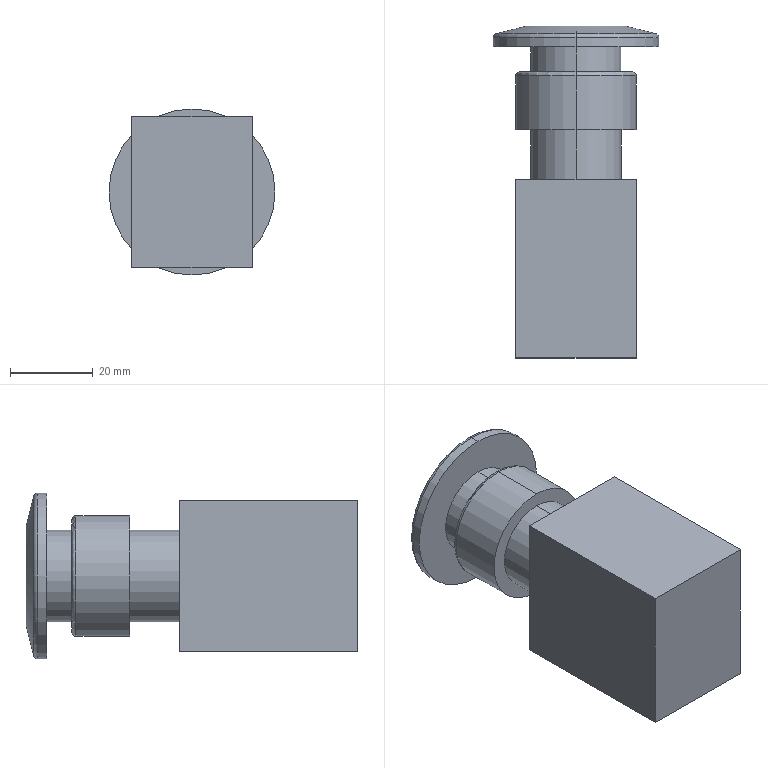Part | SolidWorks | features ICE 4, Extrusion 1, Fillet 1, RevCut 1 | 1 solid | 24 faces | box 40 x 80 x 40 mm | volume 67108 mm3 | plane 10 | cylinder 8 | torus 4 | cone 2 | commonest cylinder face diameters 22 x4 29 x2 40 x2
STEP:
#1=CARTESIAN_POINT('',(0.,-12.,-11.));
#2=VERTEX_POINT('',#1);
#3=CARTESIAN_POINT('',(0.,-12.,11.));
#4=VERTEX_POINT('',#3);
#5=CARTESIAN_POINT('',(0.,-12.,0.));
#6=DIRECTION('',(0.,-1.,0.));
#7=DIRECTION('',(0.,0.,-1.));
#8=AXIS2_PLACEMENT_3D('',#5,#6,#7);
#9=CIRCLE('',#8,11.);
#10=EDGE_CURVE('',#2,#4,#9,.T.);
#11=ORIENTED_EDGE('',*,*,#10,.F.);
#12=CARTESIAN_POINT('',(0.,0.,-11.));
#13=VERTEX_POINT('',#12);
#14=CARTESIAN_POINT('',(0.,-12.,-11.));
#15=DIRECTION('',(0.,1.,0.));
#16=VECTOR('',#15,1000.);
#17=LINE('',#14,#16);
#18=EDGE_CURVE('',#2,#13,#17,.T.);
#19=ORIENTED_EDGE('',*,*,#18,.T.);
#20=CARTESIAN_POINT('',(0.,0.,11.));
#21=VERTEX_POINT('',#20);
#22=CARTESIAN_POINT('',(0.,0.,0.));
#23=DIRECTION('',(0.,-1.,0.));
#24=DIRECTION('',(0.,0.,1.));
#25=AXIS2_PLACEMENT_3D('',#22,#23,#24);
#26=CIRCLE('',#25,11.);
#27=EDGE_CURVE('',#13,#21,#26,.T.);
#28=ORIENTED_EDGE('',*,*,#27,.T.);
#29=CARTESIAN_POINT('',(0.,-12.,11.));
#30=DIRECTION('',(0.,1.,0.));
#31=VECTOR('',#30,1000.);
#32=LINE('',#29,#31);
#33=EDGE_CURVE('',#4,#21,#32,.T.);
#34=ORIENTED_EDGE('',*,*,#33,.F.);
#35=EDGE_LOOP('',(#11,#19,#28,#34));
#36=FACE_OUTER_BOUND('',#35,.T.);
#37=CARTESIAN_POINT('',(0.,-12.,0.));
#38=DIRECTION('',(0.,1.,0.));
#39=DIRECTION('',(0.,0.,1.));
#40=AXIS2_PLACEMENT_3D('',#37,#38,#39);
#41=CYLINDRICAL_SURFACE('',#40,11.);
#42=ADVANCED_FACE('',(#36),#41,.T.);
#43=CARTESIAN_POINT('',(0.,22.219,-20.));
#44=VERTEX_POINT('',#43);
#45=CARTESIAN_POINT('',(0.,22.219,20.));
#46=VERTEX_POINT('',#45);
#47=CARTESIAN_POINT('',(0.,22.219,0.));
#48=DIRECTION('',(0.,-1.,0.));
#49=DIRECTION('',(0.,0.,1.));
#50=AXIS2_PLACEMENT_3D('',#47,#48,#49);
#51=CIRCLE('',#50,20.);
#52=EDGE_CURVE('',#44,#46,#51,.T.);
#53=ORIENTED_EDGE('',*,*,#52,.F.);
#54=CARTESIAN_POINT('',(0.,23.189,-19.243));
#55=VERTEX_POINT('',#54);
#56=CARTESIAN_POINT('',(0.,22.219,-19.));
#57=DIRECTION('',(1.,0.,0.));
#58=DIRECTION('',(0.,0.,-1.));
#59=AXIS2_PLACEMENT_3D('',#56,#57,#58);
#60=CIRCLE('',#59,1.);
#61=EDGE_CURVE('',#44,#55,#60,.T.);
#62=ORIENTED_EDGE('',*,*,#61,.T.);
#63=CARTESIAN_POINT('',(0.,23.189,19.243));
#64=VERTEX_POINT('',#63);
#65=CARTESIAN_POINT('',(0.,23.189,0.));
#66=DIRECTION('',(0.,1.,0.));
#67=DIRECTION('',(0.,0.,-1.));
#68=AXIS2_PLACEMENT_3D('',#65,#66,#67);
#69=CIRCLE('',#68,19.243);
#70=EDGE_CURVE('',#64,#55,#69,.T.);
#71=ORIENTED_EDGE('',*,*,#70,.F.);
#72=CARTESIAN_POINT('',(0.,22.219,19.));
#73=DIRECTION('',(-1.,0.,0.));
#74=DIRECTION('',(0.,0.,1.));
#75=AXIS2_PLACEMENT_3D('',#72,#73,#74);
#76=CIRCLE('',#75,1.);
#77=EDGE_CURVE('',#46,#64,#76,.T.);
#78=ORIENTED_EDGE('',*,*,#77,.F.);
#79=EDGE_LOOP('',(#53,#62,#71,#78));
#80=FACE_OUTER_BOUND('',#79,.T.);
#81=CARTESIAN_POINT('',(0.,22.219,0.));
#82=DIRECTION('',(0.,1.,0.));
#83=DIRECTION('',(0.,0.,1.));
#84=AXIS2_PLACEMENT_3D('',#81,#82,#83);
#85=TOROIDAL_SURFACE('',#84,19.,1.);
#86=ADVANCED_FACE('',(#80),#85,.T.);
#87=CARTESIAN_POINT('',(0.,13.,-14.5));
#88=VERTEX_POINT('',#87);
#89=CARTESIAN_POINT('',(0.,13.,14.5));
#90=VERTEX_POINT('',#89);
#91=CARTESIAN_POINT('',(0.,13.,0.));
#92=DIRECTION('',(0.,-1.,0.));
#93=DIRECTION('',(0.,0.,1.));
#94=AXIS2_PLACEMENT_3D('',#91,#92,#93);
#95=CIRCLE('',#94,14.5);
#96=EDGE_CURVE('',#88,#90,#95,.T.);
#97=ORIENTED_EDGE('',*,*,#96,.F.);
#98=CARTESIAN_POINT('',(0.,14.,-13.5));
#99=VERTEX_POINT('',#98);
#100=CARTESIAN_POINT('',(0.,13.,-13.5));
#101=DIRECTION('',(1.,0.,0.));
#102=DIRECTION('',(0.,0.,-1.));
#103=AXIS2_PLACEMENT_3D('',#100,#101,#102);
#104=CIRCLE('',#103,1.);
#105=EDGE_CURVE('',#88,#99,#104,.T.);
#106=ORIENTED_EDGE('',*,*,#105,.T.);
#107=CARTESIAN_POINT('',(0.,14.,13.5));
#108=VERTEX_POINT('',#107);
#109=CARTESIAN_POINT('',(0.,14.,0.));
#110=DIRECTION('',(0.,1.,0.));
#111=DIRECTION('',(0.,0.,1.));
#112=AXIS2_PLACEMENT_3D('',#109,#110,#111);
#113=CIRCLE('',#112,13.5);
#114=EDGE_CURVE('',#108,#99,#113,.T.);
#115=ORIENTED_EDGE('',*,*,#114,.F.);
#116=CARTESIAN_POINT('',(0.,13.,13.5));
#117=DIRECTION('',(-1.,0.,0.));
#118=DIRECTION('',(0.,0.,1.));
#119=AXIS2_PLACEMENT_3D('',#116,#117,#118);
#120=CIRCLE('',#119,1.);
#121=EDGE_CURVE('',#90,#108,#120,.T.);
#122=ORIENTED_EDGE('',*,*,#121,.F.);
#123=EDGE_LOOP('',(#97,#106,#115,#122));
#124=FACE_OUTER_BOUND('',#123,.T.);
#125=CARTESIAN_POINT('',(0.,13.,0.));
#126=DIRECTION('',(0.,1.,0.));
#127=DIRECTION('',(0.,0.,1.));
#128=AXIS2_PLACEMENT_3D('',#125,#126,#127);
#129=TOROIDAL_SURFACE('',#128,13.5,1.);
#130=ADVANCED_FACE('',(#124),#129,.T.);
#131=CARTESIAN_POINT('',(0.,25.,-12.));
#132=VERTEX_POINT('',#131);
#133=CARTESIAN_POINT('',(0.,25.,12.));
#134=VERTEX_POINT('',#133);
#135=CARTESIAN_POINT('',(0.,25.,0.));
#136=DIRECTION('',(0.,-1.,0.));
#137=DIRECTION('',(0.,0.,-1.));
#138=AXIS2_PLACEMENT_3D('',#135,#136,#137);
#139=CIRCLE('',#138,12.);
#140=EDGE_CURVE('',#132,#134,#139,.T.);
#141=ORIENTED_EDGE('',*,*,#140,.T.);
#142=CARTESIAN_POINT('',(0.,23.,20.));
#143=DIRECTION('',(0.,-0.2425,0.9701));
#144=VECTOR('',#143,1000.);
#145=LINE('',#142,#144);
#146=EDGE_CURVE('',#134,#64,#145,.T.);
#147=ORIENTED_EDGE('',*,*,#146,.T.);
#148=ORIENTED_EDGE('',*,*,#70,.T.);
#149=CARTESIAN_POINT('',(0.,23.,-20.));
#150=DIRECTION('',(0.,-0.2425,-0.9701));
#151=VECTOR('',#150,1000.);
#152=LINE('',#149,#151);
#153=EDGE_CURVE('',#132,#55,#152,.T.);
#154=ORIENTED_EDGE('',*,*,#153,.F.);
#155=EDGE_LOOP('',(#141,#147,#148,#154));
#156=FACE_OUTER_BOUND('',#155,.T.);
#157=CARTESIAN_POINT('',(0.,23.,0.));
#158=DIRECTION('',(0.,-1.,0.));
#159=DIRECTION('',(0.,0.,-1.));
#160=AXIS2_PLACEMENT_3D('',#157,#158,#159);
#161=CONICAL_SURFACE('',#160,20.,1.326);
#162=ADVANCED_FACE('',(#156),#161,.T.);
#163=CARTESIAN_POINT('',(0.,20.,11.));
#164=VERTEX_POINT('',#163);
#165=CARTESIAN_POINT('',(0.,20.,-11.));
#166=VERTEX_POINT('',#165);
#167=CARTESIAN_POINT('',(0.,20.,0.));
#168=DIRECTION('',(0.,1.,0.));
#169=DIRECTION('',(0.,0.,1.));
#170=AXIS2_PLACEMENT_3D('',#167,#168,#169);
#171=CIRCLE('',#170,11.);
#172=EDGE_CURVE('',#164,#166,#171,.T.);
#173=ORIENTED_EDGE('',*,*,#172,.F.);
#174=CARTESIAN_POINT('',(0.,14.,11.));
#175=VERTEX_POINT('',#174);
#176=CARTESIAN_POINT('',(0.,20.,11.));
#177=DIRECTION('',(0.,-1.,0.));
#178=VECTOR('',#177,1000.);
#179=LINE('',#176,#178);
#180=EDGE_CURVE('',#164,#175,#179,.T.);
#181=ORIENTED_EDGE('',*,*,#180,.T.);
#182=CARTESIAN_POINT('',(0.,14.,-11.));
#183=VERTEX_POINT('',#182);
#184=CARTESIAN_POINT('',(0.,14.,0.));
#185=DIRECTION('',(0.,1.,0.));
#186=DIRECTION('',(0.,0.,1.));
#187=AXIS2_PLACEMENT_3D('',#184,#185,#186);
#188=CIRCLE('',#187,11.);
#189=EDGE_CURVE('',#175,#183,#188,.T.);
#190=ORIENTED_EDGE('',*,*,#189,.T.);
#191=CARTESIAN_POINT('',(0.,20.,-11.));
#192=DIRECTION('',(0.,-1.,0.));
#193=VECTOR('',#192,1000.);
#194=LINE('',#191,#193);
#195=EDGE_CURVE('',#166,#183,#194,.T.);
#196=ORIENTED_EDGE('',*,*,#195,.F.);
#197=EDGE_LOOP('',(#173,#181,#190,#196));
#198=FACE_OUTER_BOUND('',#197,.T.);
#199=CARTESIAN_POINT('',(0.,20.,0.));
#200=DIRECTION('',(0.,-1.,0.));
#201=DIRECTION('',(0.,0.,-1.));
#202=AXIS2_PLACEMENT_3D('',#199,#200,#201);
#203=CYLINDRICAL_SURFACE('',#202,11.);
#204=ADVANCED_FACE('',(#198),#203,.T.);
#205=ORIENTED_EDGE('',*,*,#96,.T.);
#206=CARTESIAN_POINT('',(0.,0.,14.5));
#207=VERTEX_POINT('',#206);
#208=CARTESIAN_POINT('',(0.,14.,14.5));
#209=DIRECTION('',(0.,-1.,0.));
#210=VECTOR('',#209,1000.);
#211=LINE('',#208,#210);
#212=EDGE_CURVE('',#90,#207,#211,.T.);
#213=ORIENTED_EDGE('',*,*,#212,.T.);
#214=CARTESIAN_POINT('',(0.,0.,-14.5));
#215=VERTEX_POINT('',#214);
#216=CARTESIAN_POINT('',(0.,0.,0.));
#217=DIRECTION('',(0.,1.,0.));
#218=DIRECTION('',(0.,0.,1.));
#219=AXIS2_PLACEMENT_3D('',#216,#217,#218);
#220=CIRCLE('',#219,14.5);
#221=EDGE_CURVE('',#207,#215,#220,.T.);
#222=ORIENTED_EDGE('',*,*,#221,.T.);
#223=CARTESIAN_POINT('',(0.,14.,-14.5));
#224=DIRECTION('',(0.,-1.,0.));
#225=VECTOR('',#224,1000.);
#226=LINE('',#223,#225);
#227=EDGE_CURVE('',#88,#215,#226,.T.);
#228=ORIENTED_EDGE('',*,*,#227,.F.);
#229=EDGE_LOOP('',(#205,#213,#222,#228));
#230=FACE_OUTER_BOUND('',#229,.T.);
#231=CARTESIAN_POINT('',(0.,14.,0.));
#232=DIRECTION('',(0.,-1.,0.));
#233=DIRECTION('',(0.,0.,-1.));
#234=AXIS2_PLACEMENT_3D('',#231,#232,#233);
#235=CYLINDRICAL_SURFACE('',#234,14.5);
#236=ADVANCED_FACE('',(#230),#235,.T.);
#237=ORIENTED_EDGE('',*,*,#52,.T.);
#238=CARTESIAN_POINT('',(0.,20.,20.));
#239=VERTEX_POINT('',#238);
#240=CARTESIAN_POINT('',(0.,25.,20.));
#241=DIRECTION('',(0.,-1.,0.));
#242=VECTOR('',#241,1000.);
#243=LINE('',#240,#242);
#244=EDGE_CURVE('',#46,#239,#243,.T.);
#245=ORIENTED_EDGE('',*,*,#244,.T.);
#246=CARTESIAN_POINT('',(0.,20.,-20.));
#247=VERTEX_POINT('',#246);
#248=CARTESIAN_POINT('',(0.,20.,0.));
#249=DIRECTION('',(0.,1.,0.));
#250=DIRECTION('',(0.,0.,1.));
#251=AXIS2_PLACEMENT_3D('',#248,#249,#250);
#252=CIRCLE('',#251,20.);
#253=EDGE_CURVE('',#239,#247,#252,.T.);
#254=ORIENTED_EDGE('',*,*,#253,.T.);
#255=CARTESIAN_POINT('',(0.,25.,-20.));
#256=DIRECTION('',(0.,-1.,0.));
#257=VECTOR('',#256,1000.);
#258=LINE('',#255,#257);
#259=EDGE_CURVE('',#44,#247,#258,.T.);
#260=ORIENTED_EDGE('',*,*,#259,.F.);
#261=EDGE_LOOP('',(#237,#245,#254,#260));
#262=FACE_OUTER_BOUND('',#261,.T.);
#263=CARTESIAN_POINT('',(0.,25.,0.));
#264=DIRECTION('',(0.,-1.,0.));
#265=DIRECTION('',(0.,0.,-1.));
#266=AXIS2_PLACEMENT_3D('',#263,#264,#265);
#267=CYLINDRICAL_SURFACE('',#266,20.);
#268=ADVANCED_FACE('',(#262),#267,.T.);
#269=CARTESIAN_POINT('',(0.,0.,0.));
#270=DIRECTION('',(0.,1.,0.));
#271=DIRECTION('',(0.,0.,1.));
#272=AXIS2_PLACEMENT_3D('',#269,#270,#271);
#273=CIRCLE('',#272,14.5);
#274=EDGE_CURVE('',#215,#207,#273,.T.);
#275=ORIENTED_EDGE('',*,*,#274,.F.);
#276=ORIENTED_EDGE('',*,*,#221,.F.);
#277=EDGE_LOOP('',(#275,#276));
#278=FACE_OUTER_BOUND('',#277,.T.);
#279=CARTESIAN_POINT('',(0.,0.,0.));
#280=DIRECTION('',(0.,-1.,0.));
#281=DIRECTION('',(0.,0.,1.));
#282=AXIS2_PLACEMENT_3D('',#279,#280,#281);
#283=CIRCLE('',#282,11.);
#284=EDGE_CURVE('',#21,#13,#283,.T.);
#285=ORIENTED_EDGE('',*,*,#284,.F.);
#286=ORIENTED_EDGE('',*,*,#27,.F.);
#287=EDGE_LOOP('',(#285,#286));
#288=FACE_BOUND('',#287,.T.);
#289=CARTESIAN_POINT('',(0.,0.,0.));
#290=DIRECTION('',(0.,1.,0.));
#291=DIRECTION('',(0.,0.,1.));
#292=AXIS2_PLACEMENT_3D('',#289,#290,#291);
#293=PLANE('',#292);
#294=ADVANCED_FACE('',(#278,#288),#293,.F.);
#295=ORIENTED_EDGE('',*,*,#244,.F.);
#296=CARTESIAN_POINT('',(0.,22.219,0.));
#297=DIRECTION('',(0.,-1.,0.));
#298=DIRECTION('',(0.,0.,1.));
#299=AXIS2_PLACEMENT_3D('',#296,#297,#298);
#300=CIRCLE('',#299,20.);
#301=EDGE_CURVE('',#46,#44,#300,.T.);
#302=ORIENTED_EDGE('',*,*,#301,.T.);
#303=ORIENTED_EDGE('',*,*,#259,.T.);
#304=CARTESIAN_POINT('',(0.,20.,0.));
#305=DIRECTION('',(0.,1.,0.));
#306=DIRECTION('',(0.,0.,1.));
#307=AXIS2_PLACEMENT_3D('',#304,#305,#306);
#308=CIRCLE('',#307,20.);
#309=EDGE_CURVE('',#247,#239,#308,.T.);
#310=ORIENTED_EDGE('',*,*,#309,.T.);
#311=EDGE_LOOP('',(#295,#302,#303,#310));
#312=FACE_OUTER_BOUND('',#311,.T.);
#313=CARTESIAN_POINT('',(0.,25.,0.));
#314=DIRECTION('',(0.,-1.,0.));
#315=DIRECTION('',(0.,0.,-1.));
#316=AXIS2_PLACEMENT_3D('',#313,#314,#315);
#317=CYLINDRICAL_SURFACE('',#316,20.);
#318=ADVANCED_FACE('',(#312),#317,.T.);
#319=ORIENTED_EDGE('',*,*,#114,.T.);
#320=CARTESIAN_POINT('',(0.,14.,0.));
#321=DIRECTION('',(0.,1.,0.));
#322=DIRECTION('',(0.,0.,1.));
#323=AXIS2_PLACEMENT_3D('',#320,#321,#322);
#324=CIRCLE('',#323,13.5);
#325=EDGE_CURVE('',#99,#108,#324,.T.);
#326=ORIENTED_EDGE('',*,*,#325,.T.);
#327=EDGE_LOOP('',(#319,#326));
#328=FACE_OUTER_BOUND('',#327,.T.);
#329=CARTESIAN_POINT('',(0.,14.,0.));
#330=DIRECTION('',(0.,1.,0.));
#331=DIRECTION('',(0.,0.,1.));
#332=AXIS2_PLACEMENT_3D('',#329,#330,#331);
#333=CIRCLE('',#332,11.);
#334=EDGE_CURVE('',#183,#175,#333,.T.);
#335=ORIENTED_EDGE('',*,*,#334,.F.);
#336=ORIENTED_EDGE('',*,*,#189,.F.);
#337=EDGE_LOOP('',(#335,#336));
#338=FACE_BOUND('',#337,.T.);
#339=CARTESIAN_POINT('',(0.,14.,0.));
#340=DIRECTION('',(0.,1.,0.));
#341=DIRECTION('',(0.,0.,1.));
#342=AXIS2_PLACEMENT_3D('',#339,#340,#341);
#343=PLANE('',#342);
#344=ADVANCED_FACE('',(#328,#338),#343,.T.);
#345=ORIENTED_EDGE('',*,*,#212,.F.);
#346=CARTESIAN_POINT('',(0.,13.,0.));
#347=DIRECTION('',(0.,-1.,0.));
#348=DIRECTION('',(0.,0.,1.));
#349=AXIS2_PLACEMENT_3D('',#346,#347,#348);
#350=CIRCLE('',#349,14.5);
#351=EDGE_CURVE('',#90,#88,#350,.T.);
#352=ORIENTED_EDGE('',*,*,#351,.T.);
#353=ORIENTED_EDGE('',*,*,#227,.T.);
#354=ORIENTED_EDGE('',*,*,#274,.T.);
#355=EDGE_LOOP('',(#345,#352,#353,#354));
#356=FACE_OUTER_BOUND('',#355,.T.);
#357=CARTESIAN_POINT('',(0.,14.,0.));
#358=DIRECTION('',(0.,-1.,0.));
#359=DIRECTION('',(0.,0.,-1.));
#360=AXIS2_PLACEMENT_3D('',#357,#358,#359);
#361=CYLINDRICAL_SURFACE('',#360,14.5);
#362=ADVANCED_FACE('',(#356),#361,.T.);
#363=ORIENTED_EDGE('',*,*,#180,.F.);
#364=CARTESIAN_POINT('',(0.,20.,0.));
#365=DIRECTION('',(0.,1.,0.));
#366=DIRECTION('',(0.,0.,1.));
#367=AXIS2_PLACEMENT_3D('',#364,#365,#366);
#368=CIRCLE('',#367,11.);
#369=EDGE_CURVE('',#166,#164,#368,.T.);
#370=ORIENTED_EDGE('',*,*,#369,.F.);
#371=ORIENTED_EDGE('',*,*,#195,.T.);
#372=ORIENTED_EDGE('',*,*,#334,.T.);
#373=EDGE_LOOP('',(#363,#370,#371,#372));
#374=FACE_OUTER_BOUND('',#373,.T.);
#375=CARTESIAN_POINT('',(0.,20.,0.));
#376=DIRECTION('',(0.,-1.,0.));
#377=DIRECTION('',(0.,0.,-1.));
#378=AXIS2_PLACEMENT_3D('',#375,#376,#377);
#379=CYLINDRICAL_SURFACE('',#378,11.);
#380=ADVANCED_FACE('',(#374),#379,.T.);
#381=ORIENTED_EDGE('',*,*,#309,.F.);
#382=ORIENTED_EDGE('',*,*,#253,.F.);
#383=EDGE_LOOP('',(#381,#382));
#384=FACE_OUTER_BOUND('',#383,.T.);
#385=ORIENTED_EDGE('',*,*,#369,.T.);
#386=ORIENTED_EDGE('',*,*,#172,.T.);
#387=EDGE_LOOP('',(#385,#386));
#388=FACE_BOUND('',#387,.T.);
#389=CARTESIAN_POINT('',(0.,20.,0.));
#390=DIRECTION('',(0.,1.,0.));
#391=DIRECTION('',(0.,0.,1.));
#392=AXIS2_PLACEMENT_3D('',#389,#390,#391);
#393=PLANE('',#392);
#394=ADVANCED_FACE('',(#384,#388),#393,.F.);
#395=ORIENTED_EDGE('',*,*,#146,.F.);
#396=CARTESIAN_POINT('',(0.,25.,0.));
#397=DIRECTION('',(0.,-1.,0.));
#398=DIRECTION('',(0.,0.,-1.));
#399=AXIS2_PLACEMENT_3D('',#396,#397,#398);
#400=CIRCLE('',#399,12.);
#401=EDGE_CURVE('',#134,#132,#400,.T.);
#402=ORIENTED_EDGE('',*,*,#401,.T.);
#403=ORIENTED_EDGE('',*,*,#153,.T.);
#404=CARTESIAN_POINT('',(0.,23.189,0.));
#405=DIRECTION('',(0.,1.,0.));
#406=DIRECTION('',(0.,0.,-1.));
#407=AXIS2_PLACEMENT_3D('',#404,#405,#406);
#408=CIRCLE('',#407,19.243);
#409=EDGE_CURVE('',#55,#64,#408,.T.);
#410=ORIENTED_EDGE('',*,*,#409,.T.);
#411=EDGE_LOOP('',(#395,#402,#403,#410));
#412=FACE_OUTER_BOUND('',#411,.T.);
#413=CARTESIAN_POINT('',(0.,23.,0.));
#414=DIRECTION('',(0.,-1.,0.));
#415=DIRECTION('',(0.,0.,-1.));
#416=AXIS2_PLACEMENT_3D('',#413,#414,#415);
#417=CONICAL_SURFACE('',#416,20.,1.326);
#418=ADVANCED_FACE('',(#412),#417,.T.);
#419=ORIENTED_EDGE('',*,*,#140,.F.);
#420=ORIENTED_EDGE('',*,*,#401,.F.);
#421=EDGE_LOOP('',(#419,#420));
#422=FACE_OUTER_BOUND('',#421,.T.);
#423=CARTESIAN_POINT('',(0.,25.,0.));
#424=DIRECTION('',(0.,1.,0.));
#425=DIRECTION('',(0.,0.,1.));
#426=AXIS2_PLACEMENT_3D('',#423,#424,#425);
#427=PLANE('',#426);
#428=ADVANCED_FACE('',(#422),#427,.T.);
#429=ORIENTED_EDGE('',*,*,#105,.F.);
#430=ORIENTED_EDGE('',*,*,#351,.F.);
#431=ORIENTED_EDGE('',*,*,#121,.T.);
#432=ORIENTED_EDGE('',*,*,#325,.F.);
#433=EDGE_LOOP('',(#429,#430,#431,#432));
#434=FACE_OUTER_BOUND('',#433,.T.);
#435=CARTESIAN_POINT('',(0.,13.,0.));
#436=DIRECTION('',(0.,1.,0.));
#437=DIRECTION('',(0.,0.,1.));
#438=AXIS2_PLACEMENT_3D('',#435,#436,#437);
#439=TOROIDAL_SURFACE('',#438,13.5,1.);
#440=ADVANCED_FACE('',(#434),#439,.T.);
#441=ORIENTED_EDGE('',*,*,#61,.F.);
#442=ORIENTED_EDGE('',*,*,#301,.F.);
#443=ORIENTED_EDGE('',*,*,#77,.T.);
#444=ORIENTED_EDGE('',*,*,#409,.F.);
#445=EDGE_LOOP('',(#441,#442,#443,#444));
#446=FACE_OUTER_BOUND('',#445,.T.);
#447=CARTESIAN_POINT('',(0.,22.219,0.));
#448=DIRECTION('',(0.,1.,0.));
#449=DIRECTION('',(0.,0.,1.));
#450=AXIS2_PLACEMENT_3D('',#447,#448,#449);
#451=TOROIDAL_SURFACE('',#450,19.,1.);
#452=ADVANCED_FACE('',(#446),#451,.T.);
#453=ORIENTED_EDGE('',*,*,#18,.F.);
#454=CARTESIAN_POINT('',(0.,-12.,0.));
#455=DIRECTION('',(0.,-1.,0.));
#456=DIRECTION('',(0.,0.,-1.));
#457=AXIS2_PLACEMENT_3D('',#454,#455,#456);
#458=CIRCLE('',#457,11.);
#459=EDGE_CURVE('',#4,#2,#458,.T.);
#460=ORIENTED_EDGE('',*,*,#459,.F.);
#461=ORIENTED_EDGE('',*,*,#33,.T.);
#462=ORIENTED_EDGE('',*,*,#284,.T.);
#463=EDGE_LOOP('',(#453,#460,#461,#462));
#464=FACE_OUTER_BOUND('',#463,.T.);
#465=CARTESIAN_POINT('',(0.,-12.,0.));
#466=DIRECTION('',(0.,1.,0.));
#467=DIRECTION('',(0.,0.,1.));
#468=AXIS2_PLACEMENT_3D('',#465,#466,#467);
#469=CYLINDRICAL_SURFACE('',#468,11.);
#470=ADVANCED_FACE('',(#464),#469,.T.);
#471=CARTESIAN_POINT('',(14.5,-12.,-18.3));
#472=VERTEX_POINT('',#471);
#473=CARTESIAN_POINT('',(14.5,-12.,18.3));
#474=VERTEX_POINT('',#473);
#475=CARTESIAN_POINT('',(14.5,-12.,-18.3));
#476=DIRECTION('',(0.,0.,1.));
#477=VECTOR('',#476,1000.);
#478=LINE('',#475,#477);
#479=EDGE_CURVE('',#472,#474,#478,.T.);
#480=ORIENTED_EDGE('',*,*,#479,.F.);
#481=CARTESIAN_POINT('',(-14.5,-12.,-18.3));
#482=VERTEX_POINT('',#481);
#483=CARTESIAN_POINT('',(-14.5,-12.,-18.3));
#484=DIRECTION('',(1.,0.,0.));
#485=VECTOR('',#484,1000.);
#486=LINE('',#483,#485);
#487=EDGE_CURVE('',#482,#472,#486,.T.);
#488=ORIENTED_EDGE('',*,*,#487,.F.);
#489=CARTESIAN_POINT('',(-14.5,-12.,18.3));
#490=VERTEX_POINT('',#489);
#491=CARTESIAN_POINT('',(-14.5,-12.,-18.3));
#492=DIRECTION('',(0.,0.,-1.));
#493=VECTOR('',#492,1000.);
#494=LINE('',#491,#493);
#495=EDGE_CURVE('',#490,#482,#494,.T.);
#496=ORIENTED_EDGE('',*,*,#495,.F.);
#497=CARTESIAN_POINT('',(-14.5,-12.,18.3));
#498=DIRECTION('',(-1.,0.,0.));
#499=VECTOR('',#498,1000.);
#500=LINE('',#497,#499);
#501=EDGE_CURVE('',#474,#490,#500,.T.);
#502=ORIENTED_EDGE('',*,*,#501,.F.);
#503=EDGE_LOOP('',(#480,#488,#496,#502));
#504=FACE_OUTER_BOUND('',#503,.T.);
#505=ORIENTED_EDGE('',*,*,#459,.T.);
#506=ORIENTED_EDGE('',*,*,#10,.T.);
#507=EDGE_LOOP('',(#505,#506));
#508=FACE_BOUND('',#507,.T.);
#509=CARTESIAN_POINT('',(14.5,-12.,18.3));
#510=DIRECTION('',(0.,1.,0.));
#511=DIRECTION('',(0.,0.,1.));
#512=AXIS2_PLACEMENT_3D('',#509,#510,#511);
#513=PLANE('',#512);
#514=ADVANCED_FACE('',(#504,#508),#513,.T.);
#515=ORIENTED_EDGE('',*,*,#479,.T.);
#516=CARTESIAN_POINT('',(14.5,-55.,18.3));
#517=VERTEX_POINT('',#516);
#518=CARTESIAN_POINT('',(14.5,-55.,18.3));
#519=DIRECTION('',(0.,1.,0.));
#520=VECTOR('',#519,1000.);
#521=LINE('',#518,#520);
#522=EDGE_CURVE('',#517,#474,#521,.T.);
#523=ORIENTED_EDGE('',*,*,#522,.F.);
#524=CARTESIAN_POINT('',(14.5,-55.,-18.3));
#525=VERTEX_POINT('',#524);
#526=CARTESIAN_POINT('',(14.5,-55.,-18.3));
#527=DIRECTION('',(0.,0.,1.));
#528=VECTOR('',#527,1000.);
#529=LINE('',#526,#528);
#530=EDGE_CURVE('',#525,#517,#529,.T.);
#531=ORIENTED_EDGE('',*,*,#530,.F.);
#532=CARTESIAN_POINT('',(14.5,-55.,-18.3));
#533=DIRECTION('',(0.,1.,0.));
#534=VECTOR('',#533,1000.);
#535=LINE('',#532,#534);
#536=EDGE_CURVE('',#525,#472,#535,.T.);
#537=ORIENTED_EDGE('',*,*,#536,.T.);
#538=EDGE_LOOP('',(#515,#523,#531,#537));
#539=FACE_OUTER_BOUND('',#538,.T.);
#540=CARTESIAN_POINT('',(14.5,-55.,-18.3));
#541=DIRECTION('',(-1.,0.,0.));
#542=DIRECTION('',(0.,0.,1.));
#543=AXIS2_PLACEMENT_3D('',#540,#541,#542);
#544=PLANE('',#543);
#545=ADVANCED_FACE('',(#539),#544,.F.);
#546=ORIENTED_EDGE('',*,*,#501,.T.);
#547=CARTESIAN_POINT('',(-14.5,-55.,18.3));
#548=VERTEX_POINT('',#547);
#549=CARTESIAN_POINT('',(-14.5,-55.,18.3));
#550=DIRECTION('',(0.,1.,0.));
#551=VECTOR('',#550,1000.);
#552=LINE('',#549,#551);
#553=EDGE_CURVE('',#548,#490,#552,.T.);
#554=ORIENTED_EDGE('',*,*,#553,.F.);
#555=CARTESIAN_POINT('',(-14.5,-55.,18.3));
#556=DIRECTION('',(-1.,0.,0.));
#557=VECTOR('',#556,1000.);
#558=LINE('',#555,#557);
#559=EDGE_CURVE('',#517,#548,#558,.T.);
#560=ORIENTED_EDGE('',*,*,#559,.F.);
#561=ORIENTED_EDGE('',*,*,#522,.T.);
#562=EDGE_LOOP('',(#546,#554,#560,#561));
#563=FACE_OUTER_BOUND('',#562,.T.);
#564=CARTESIAN_POINT('',(-14.5,-55.,18.3));
#565=DIRECTION('',(0.,0.,-1.));
#566=DIRECTION('',(-1.,0.,0.));
#567=AXIS2_PLACEMENT_3D('',#564,#565,#566);
#568=PLANE('',#567);
#569=ADVANCED_FACE('',(#563),#568,.F.);
#570=ORIENTED_EDGE('',*,*,#495,.T.);
#571=CARTESIAN_POINT('',(-14.5,-55.,-18.3));
#572=VERTEX_POINT('',#571);
#573=CARTESIAN_POINT('',(-14.5,-55.,-18.3));
#574=DIRECTION('',(0.,1.,0.));
#575=VECTOR('',#574,1000.);
#576=LINE('',#573,#575);
#577=EDGE_CURVE('',#572,#482,#576,.T.);
#578=ORIENTED_EDGE('',*,*,#577,.F.);
#579=CARTESIAN_POINT('',(-14.5,-55.,-18.3));
#580=DIRECTION('',(0.,0.,-1.));
#581=VECTOR('',#580,1000.);
#582=LINE('',#579,#581);
#583=EDGE_CURVE('',#548,#572,#582,.T.);
#584=ORIENTED_EDGE('',*,*,#583,.F.);
#585=ORIENTED_EDGE('',*,*,#553,.T.);
#586=EDGE_LOOP('',(#570,#578,#584,#585));
#587=FACE_OUTER_BOUND('',#586,.T.);
#588=CARTESIAN_POINT('',(-14.5,-55.,-18.3));
#589=DIRECTION('',(1.,0.,0.));
#590=DIRECTION('',(0.,0.,-1.));
#591=AXIS2_PLACEMENT_3D('',#588,#589,#590);
#592=PLANE('',#591);
#593=ADVANCED_FACE('',(#587),#592,.F.);
#594=ORIENTED_EDGE('',*,*,#487,.T.);
#595=ORIENTED_EDGE('',*,*,#536,.F.);
#596=CARTESIAN_POINT('',(-14.5,-55.,-18.3));
#597=DIRECTION('',(1.,0.,0.));
#598=VECTOR('',#597,1000.);
#599=LINE('',#596,#598);
#600=EDGE_CURVE('',#572,#525,#599,.T.);
#601=ORIENTED_EDGE('',*,*,#600,.F.);
#602=ORIENTED_EDGE('',*,*,#577,.T.);
#603=EDGE_LOOP('',(#594,#595,#601,#602));
#604=FACE_OUTER_BOUND('',#603,.T.);
#605=CARTESIAN_POINT('',(-14.5,-55.,-18.3));
#606=DIRECTION('',(0.,0.,1.));
#607=DIRECTION('',(1.,0.,0.));
#608=AXIS2_PLACEMENT_3D('',#605,#606,#607);
#609=PLANE('',#608);
#610=ADVANCED_FACE('',(#604),#609,.F.);
#611=ORIENTED_EDGE('',*,*,#530,.T.);
#612=ORIENTED_EDGE('',*,*,#559,.T.);
#613=ORIENTED_EDGE('',*,*,#583,.T.);
#614=ORIENTED_EDGE('',*,*,#600,.T.);
#615=EDGE_LOOP('',(#611,#612,#613,#614));
#616=FACE_OUTER_BOUND('',#615,.T.);
#617=CARTESIAN_POINT('',(14.5,-55.,18.3));
#618=DIRECTION('',(0.,1.,0.));
#619=DIRECTION('',(0.,0.,1.));
#620=AXIS2_PLACEMENT_3D('',#617,#618,#619);
#621=PLANE('',#620);
#622=ADVANCED_FACE('',(#616),#621,.F.);
#623=CLOSED_SHELL('',(#42,#86,#130,#162,#204,#236,#268,#294,#318,#344,#362,#380,#394,#418,#428,#440,#452,#470,#514,#545,#569,#593,#610,#622));
#624=MANIFOLD_SOLID_BREP('',#623);
#625=CARTESIAN_POINT('',(0.,0.,0.));
#626=DIRECTION('',(0.,0.,1.));
#627=DIRECTION('',(1.,0.,0.));
#628=AXIS2_PLACEMENT_3D('',#625,#626,#627);
#629=(LENGTH_UNIT()NAMED_UNIT(*)SI_UNIT(.MILLI.,.METRE.));
#630=UNCERTAINTY_MEASURE_WITH_UNIT(LENGTH_MEASURE(0.00001),#629,'','');
#631=(NAMED_UNIT(*)PLANE_ANGLE_UNIT()SI_UNIT($,.RADIAN.));
#632=(NAMED_UNIT(*)SI_UNIT($,.STERADIAN.)SOLID_ANGLE_UNIT());
#633=(GEOMETRIC_REPRESENTATION_CONTEXT(3)GLOBAL_UNCERTAINTY_ASSIGNED_CONTEXT((#630))GLOBAL_UNIT_ASSIGNED_CONTEXT((#629,#631,#632))REPRESENTATION_CONTEXT('',''));
#634=ADVANCED_BREP_SHAPE_REPRESENTATION('',(#624,#628),#633);